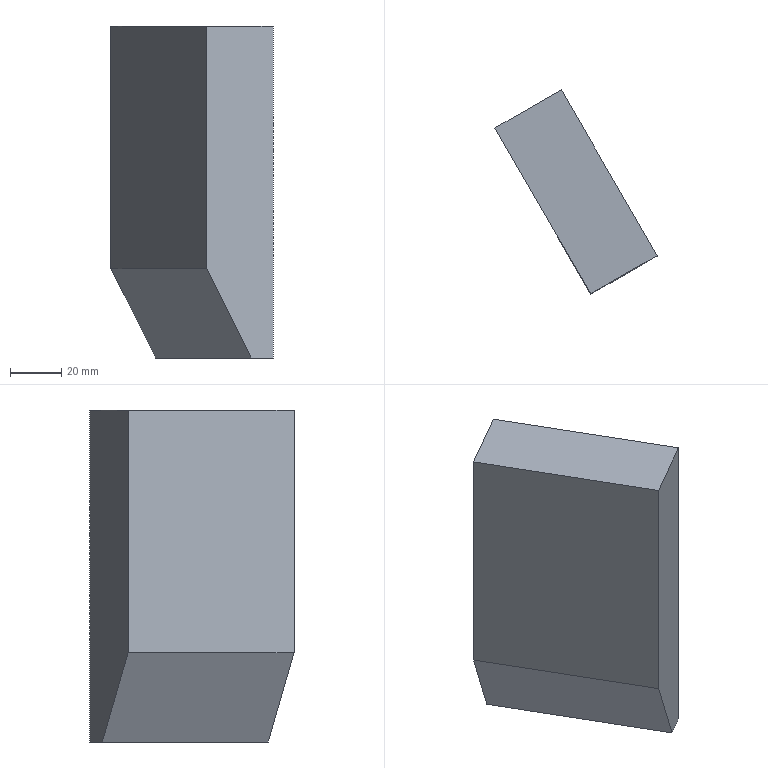Part | NX | features solid 2 | 1 solid | 7 faces | box 63.481 x 79.952 x 130 mm | volume 265978 mm3 | plane 7
STEP:
#1=CARTESIAN_POINT('',(-1191.402,-6.76,139.));
#2=VERTEX_POINT('',#1);
#3=CARTESIAN_POINT('',(-1153.902,-71.712,139.));
#4=VERTEX_POINT('',#3);
#5=CARTESIAN_POINT('',(-1114.152,-140.561,139.));
#6=DIRECTION('',(0.5,-0.866,0.));
#7=VECTOR('',#6,1000.);
#8=LINE('',#5,#7);
#9=EDGE_CURVE('',#2,#4,#8,.T.);
#10=ORIENTED_EDGE('',*,*,#9,.F.);
#11=CARTESIAN_POINT('',(-1191.402,-6.76,44.));
#12=VERTEX_POINT('',#11);
#13=CARTESIAN_POINT('',(-1191.402,-6.76,139.));
#14=DIRECTION('',(0.,0.,1.));
#15=VECTOR('',#14,1000.);
#16=LINE('',#13,#15);
#17=EDGE_CURVE('',#2,#12,#16,.F.);
#18=ORIENTED_EDGE('',*,*,#17,.T.);
#19=CARTESIAN_POINT('',(-1153.902,-71.712,44.));
#20=VERTEX_POINT('',#19);
#21=CARTESIAN_POINT('',(-1114.152,-140.561,44.));
#22=DIRECTION('',(0.5,-0.866,0.));
#23=VECTOR('',#22,1000.);
#24=LINE('',#21,#23);
#25=EDGE_CURVE('',#12,#20,#24,.T.);
#26=ORIENTED_EDGE('',*,*,#25,.T.);
#27=CARTESIAN_POINT('',(-1153.902,-71.712,219.));
#28=DIRECTION('',(0.,0.,1.));
#29=VECTOR('',#28,1000.);
#30=LINE('',#27,#29);
#31=EDGE_CURVE('',#20,#4,#30,.T.);
#32=ORIENTED_EDGE('',*,*,#31,.T.);
#33=EDGE_LOOP('',(#10,#18,#26,#32));
#34=FACE_BOUND('',#33,.T.);
#35=CARTESIAN_POINT('',(-1114.152,-140.561,139.));
#36=DIRECTION('',(-0.866,-0.5,0.));
#37=DIRECTION('',(0.5,-0.866,0.));
#38=AXIS2_PLACEMENT_3D('',#35,#36,#37);
#39=PLANE('',#38);
#40=ADVANCED_FACE('',(#34),#39,.T.);
#41=ORIENTED_EDGE('',*,*,#25,.F.);
#42=CARTESIAN_POINT('',(-1173.902,3.343,9.));
#43=VERTEX_POINT('',#42);
#44=CARTESIAN_POINT('',(-1191.402,-6.76,44.));
#45=DIRECTION('',(-0.433,-0.25,0.866));
#46=VECTOR('',#45,1000.);
#47=LINE('',#44,#46);
#48=EDGE_CURVE('',#12,#43,#47,.F.);
#49=ORIENTED_EDGE('',*,*,#48,.T.);
#50=CARTESIAN_POINT('',(-1136.402,-61.609,9.));
#51=VERTEX_POINT('',#50);
#52=CARTESIAN_POINT('',(-1096.652,-130.458,9.));
#53=DIRECTION('',(-0.5,0.866,0.));
#54=VECTOR('',#53,1000.);
#55=LINE('',#52,#54);
#56=EDGE_CURVE('',#51,#43,#55,.T.);
#57=ORIENTED_EDGE('',*,*,#56,.F.);
#58=CARTESIAN_POINT('',(-1214.115,-106.476,164.425));
#59=DIRECTION('',(-0.433,-0.25,0.866));
#60=VECTOR('',#59,1000.);
#61=LINE('',#58,#60);
#62=EDGE_CURVE('',#51,#20,#61,.T.);
#63=ORIENTED_EDGE('',*,*,#62,.T.);
#64=EDGE_LOOP('',(#41,#49,#57,#63));
#65=FACE_BOUND('',#64,.T.);
#66=CARTESIAN_POINT('',(-1114.152,-140.561,44.));
#67=DIRECTION('',(-0.75,-0.433,-0.5));
#68=DIRECTION('',(-0.433,-0.25,0.866));
#69=AXIS2_PLACEMENT_3D('',#66,#67,#68);
#70=PLANE('',#69);
#71=ADVANCED_FACE('',(#65),#70,.T.);
#72=CARTESIAN_POINT('',(-1127.921,-56.712,9.));
#73=VERTEX_POINT('',#72);
#74=CARTESIAN_POINT('',(-1127.921,-56.712,139.));
#75=VERTEX_POINT('',#74);
#76=CARTESIAN_POINT('',(-1127.921,-56.712,9.));
#77=DIRECTION('',(0.,0.,1.));
#78=VECTOR('',#77,1000.);
#79=LINE('',#76,#78);
#80=EDGE_CURVE('',#73,#75,#79,.T.);
#81=ORIENTED_EDGE('',*,*,#80,.F.);
#82=CARTESIAN_POINT('',(-1165.421,8.24,9.));
#83=VERTEX_POINT('',#82);
#84=CARTESIAN_POINT('',(-1088.171,-125.561,9.));
#85=DIRECTION('',(0.5,-0.866,0.));
#86=VECTOR('',#85,1000.);
#87=LINE('',#84,#86);
#88=EDGE_CURVE('',#83,#73,#87,.T.);
#89=ORIENTED_EDGE('',*,*,#88,.F.);
#90=CARTESIAN_POINT('',(-1165.421,8.24,139.));
#91=VERTEX_POINT('',#90);
#92=CARTESIAN_POINT('',(-1165.421,8.24,219.));
#93=DIRECTION('',(0.,0.,1.));
#94=VECTOR('',#93,1000.);
#95=LINE('',#92,#94);
#96=EDGE_CURVE('',#91,#83,#95,.F.);
#97=ORIENTED_EDGE('',*,*,#96,.F.);
#98=CARTESIAN_POINT('',(-1088.171,-125.561,139.));
#99=DIRECTION('',(-0.5,0.866,0.));
#100=VECTOR('',#99,1000.);
#101=LINE('',#98,#100);
#102=EDGE_CURVE('',#75,#91,#101,.T.);
#103=ORIENTED_EDGE('',*,*,#102,.F.);
#104=EDGE_LOOP('',(#81,#89,#97,#103));
#105=FACE_BOUND('',#104,.T.);
#106=CARTESIAN_POINT('',(-1088.171,-125.561,9.));
#107=DIRECTION('',(0.866,0.5,0.));
#108=DIRECTION('',(0.,0.,-1.));
#109=AXIS2_PLACEMENT_3D('',#106,#107,#108);
#110=PLANE('',#109);
#111=ADVANCED_FACE('',(#105),#110,.T.);
#112=CARTESIAN_POINT('',(-1165.421,8.24,139.));
#113=DIRECTION('',(0.866,0.5,0.));
#114=VECTOR('',#113,1000.);
#115=LINE('',#112,#114);
#116=EDGE_CURVE('',#91,#2,#115,.F.);
#117=ORIENTED_EDGE('',*,*,#116,.T.);
#118=ORIENTED_EDGE('',*,*,#9,.T.);
#119=CARTESIAN_POINT('',(-1127.921,-56.712,139.));
#120=DIRECTION('',(-0.866,-0.5,0.));
#121=VECTOR('',#120,1000.);
#122=LINE('',#119,#121);
#123=EDGE_CURVE('',#75,#4,#122,.T.);
#124=ORIENTED_EDGE('',*,*,#123,.F.);
#125=ORIENTED_EDGE('',*,*,#102,.T.);
#126=EDGE_LOOP('',(#117,#118,#124,#125));
#127=FACE_BOUND('',#126,.T.);
#128=CARTESIAN_POINT('',(-1088.171,-125.561,139.));
#129=DIRECTION('',(0.,0.,1.));
#130=DIRECTION('',(0.5,-0.866,0.));
#131=AXIS2_PLACEMENT_3D('',#128,#129,#130);
#132=PLANE('',#131);
#133=ADVANCED_FACE('',(#127),#132,.T.);
#134=CARTESIAN_POINT('',(-1136.402,-61.609,9.));
#135=DIRECTION('',(0.866,0.5,0.));
#136=VECTOR('',#135,1000.);
#137=LINE('',#134,#136);
#138=EDGE_CURVE('',#51,#73,#137,.T.);
#139=ORIENTED_EDGE('',*,*,#138,.F.);
#140=ORIENTED_EDGE('',*,*,#56,.T.);
#141=CARTESIAN_POINT('',(-1173.902,3.343,9.));
#142=DIRECTION('',(-0.866,-0.5,0.));
#143=VECTOR('',#142,1000.);
#144=LINE('',#141,#143);
#145=EDGE_CURVE('',#43,#83,#144,.F.);
#146=ORIENTED_EDGE('',*,*,#145,.T.);
#147=ORIENTED_EDGE('',*,*,#88,.T.);
#148=EDGE_LOOP('',(#139,#140,#146,#147));
#149=FACE_BOUND('',#148,.T.);
#150=CARTESIAN_POINT('',(-1096.652,-130.458,9.));
#151=DIRECTION('',(0.,0.,-1.));
#152=DIRECTION('',(-0.5,0.866,0.));
#153=AXIS2_PLACEMENT_3D('',#150,#151,#152);
#154=PLANE('',#153);
#155=ADVANCED_FACE('',(#149),#154,.T.);
#156=ORIENTED_EDGE('',*,*,#123,.T.);
#157=ORIENTED_EDGE('',*,*,#31,.F.);
#158=ORIENTED_EDGE('',*,*,#62,.F.);
#159=ORIENTED_EDGE('',*,*,#138,.T.);
#160=ORIENTED_EDGE('',*,*,#80,.T.);
#161=EDGE_LOOP('',(#156,#157,#158,#159,#160));
#162=FACE_BOUND('',#161,.T.);
#163=CARTESIAN_POINT('',(-1132.252,-59.212,219.));
#164=DIRECTION('',(-0.5,0.866,0.));
#165=DIRECTION('',(0.,0.,-1.));
#166=AXIS2_PLACEMENT_3D('',#163,#164,#165);
#167=PLANE('',#166);
#168=ADVANCED_FACE('',(#162),#167,.F.);
#169=ORIENTED_EDGE('',*,*,#17,.F.);
#170=ORIENTED_EDGE('',*,*,#116,.F.);
#171=ORIENTED_EDGE('',*,*,#96,.T.);
#172=ORIENTED_EDGE('',*,*,#145,.F.);
#173=ORIENTED_EDGE('',*,*,#48,.F.);
#174=EDGE_LOOP('',(#169,#170,#171,#172,#173));
#175=FACE_BOUND('',#174,.T.);
#176=CARTESIAN_POINT('',(-1169.752,5.74,219.));
#177=DIRECTION('',(0.5,-0.866,0.));
#178=DIRECTION('',(0.,0.,-1.));
#179=AXIS2_PLACEMENT_3D('',#176,#177,#178);
#180=PLANE('',#179);
#181=ADVANCED_FACE('',(#175),#180,.F.);
#182=CLOSED_SHELL('',(#40,#71,#111,#133,#155,#168,#181));
#183=MANIFOLD_SOLID_BREP('',#182);
#184=(LENGTH_UNIT()NAMED_UNIT(*)SI_UNIT(.MILLI.,.METRE.));
#185=UNCERTAINTY_MEASURE_WITH_UNIT(LENGTH_MEASURE(0.00001),#184,'','');
#186=(NAMED_UNIT(*)PLANE_ANGLE_UNIT()SI_UNIT($,.RADIAN.));
#187=(NAMED_UNIT(*)SI_UNIT($,.STERADIAN.)SOLID_ANGLE_UNIT());
#188=(GEOMETRIC_REPRESENTATION_CONTEXT(3)GLOBAL_UNCERTAINTY_ASSIGNED_CONTEXT((#185))GLOBAL_UNIT_ASSIGNED_CONTEXT((#184,#186,#187))REPRESENTATION_CONTEXT('',''));
#189=ADVANCED_BREP_SHAPE_REPRESENTATION('',(#183),#188);